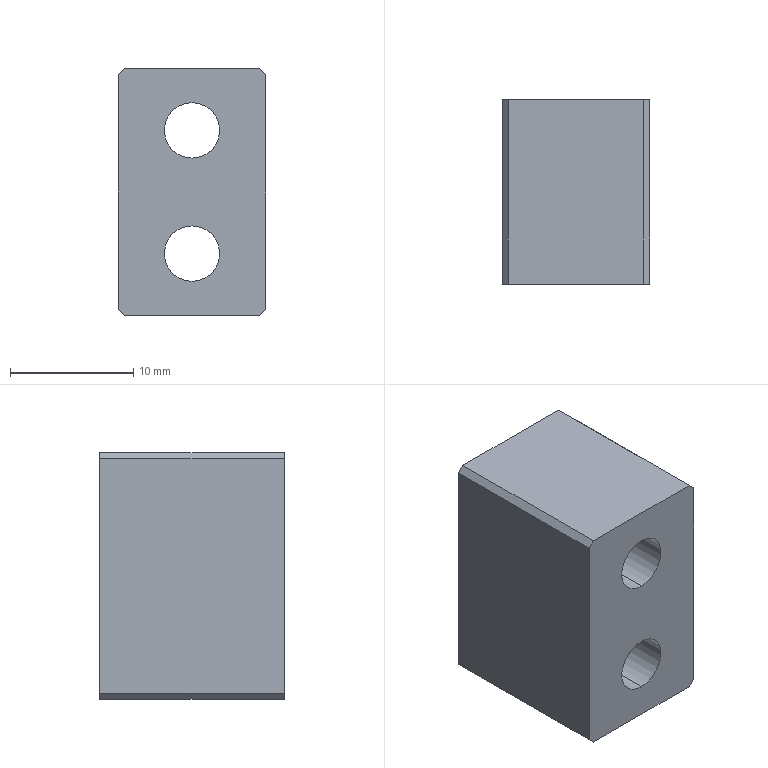Part | SolidWorks | features Chamfer 1, Extrusion 1, HoleWzd 1 | 1 solid | 20 faces | box 12 x 15 x 20 mm | volume 2799 mm3 | plane 12 | cylinder 8 | commonest cylinder face diameters 4.5 x4 8 x4
STEP:
#1=CARTESIAN_POINT('',(0.,10.4,-9.));
#2=VERTEX_POINT('',#1);
#3=CARTESIAN_POINT('',(0.,10.4,-1.));
#4=VERTEX_POINT('',#3);
#5=CARTESIAN_POINT('',(0.,10.4,-5.));
#6=DIRECTION('',(0.,1.,0.));
#7=DIRECTION('',(0.,0.,1.));
#8=AXIS2_PLACEMENT_3D('',#5,#6,#7);
#9=CIRCLE('',#8,4.);
#10=EDGE_CURVE('',#2,#4,#9,.T.);
#11=ORIENTED_EDGE('',*,*,#10,.F.);
#12=CARTESIAN_POINT('',(0.,15.,-9.));
#13=VERTEX_POINT('',#12);
#14=CARTESIAN_POINT('',(0.,15.,-9.));
#15=DIRECTION('',(0.,1.,0.));
#16=VECTOR('',#15,1000.);
#17=LINE('',#14,#16);
#18=EDGE_CURVE('',#2,#13,#17,.T.);
#19=ORIENTED_EDGE('',*,*,#18,.T.);
#20=CARTESIAN_POINT('',(0.,15.,-1.));
#21=VERTEX_POINT('',#20);
#22=CARTESIAN_POINT('',(0.,15.,-5.));
#23=DIRECTION('',(0.,1.,0.));
#24=DIRECTION('',(0.,0.,1.));
#25=AXIS2_PLACEMENT_3D('',#22,#23,#24);
#26=CIRCLE('',#25,4.);
#27=EDGE_CURVE('',#13,#21,#26,.T.);
#28=ORIENTED_EDGE('',*,*,#27,.T.);
#29=CARTESIAN_POINT('',(0.,15.,-1.));
#30=DIRECTION('',(0.,1.,0.));
#31=VECTOR('',#30,1000.);
#32=LINE('',#29,#31);
#33=EDGE_CURVE('',#4,#21,#32,.T.);
#34=ORIENTED_EDGE('',*,*,#33,.F.);
#35=EDGE_LOOP('',(#11,#19,#28,#34));
#36=FACE_OUTER_BOUND('',#35,.T.);
#37=CARTESIAN_POINT('',(0.,15.,-5.));
#38=DIRECTION('',(0.,1.,0.));
#39=DIRECTION('',(0.,0.,1.));
#40=AXIS2_PLACEMENT_3D('',#37,#38,#39);
#41=CYLINDRICAL_SURFACE('',#40,4.);
#42=ADVANCED_FACE('',(#36),#41,.F.);
#43=CARTESIAN_POINT('',(0.,0.,-7.25));
#44=VERTEX_POINT('',#43);
#45=CARTESIAN_POINT('',(0.,0.,-2.75));
#46=VERTEX_POINT('',#45);
#47=CARTESIAN_POINT('',(0.,0.,-5.));
#48=DIRECTION('',(0.,1.,0.));
#49=DIRECTION('',(0.,0.,1.));
#50=AXIS2_PLACEMENT_3D('',#47,#48,#49);
#51=CIRCLE('',#50,2.25);
#52=EDGE_CURVE('',#44,#46,#51,.T.);
#53=ORIENTED_EDGE('',*,*,#52,.F.);
#54=CARTESIAN_POINT('',(0.,10.4,-7.25));
#55=VERTEX_POINT('',#54);
#56=CARTESIAN_POINT('',(0.,15.,-7.25));
#57=DIRECTION('',(0.,1.,0.));
#58=VECTOR('',#57,1000.);
#59=LINE('',#56,#58);
#60=EDGE_CURVE('',#44,#55,#59,.T.);
#61=ORIENTED_EDGE('',*,*,#60,.T.);
#62=CARTESIAN_POINT('',(0.,10.4,-2.75));
#63=VERTEX_POINT('',#62);
#64=CARTESIAN_POINT('',(0.,10.4,-5.));
#65=DIRECTION('',(0.,1.,0.));
#66=DIRECTION('',(0.,0.,1.));
#67=AXIS2_PLACEMENT_3D('',#64,#65,#66);
#68=CIRCLE('',#67,2.25);
#69=EDGE_CURVE('',#55,#63,#68,.T.);
#70=ORIENTED_EDGE('',*,*,#69,.T.);
#71=CARTESIAN_POINT('',(0.,15.,-2.75));
#72=DIRECTION('',(0.,1.,0.));
#73=VECTOR('',#72,1000.);
#74=LINE('',#71,#73);
#75=EDGE_CURVE('',#46,#63,#74,.T.);
#76=ORIENTED_EDGE('',*,*,#75,.F.);
#77=EDGE_LOOP('',(#53,#61,#70,#76));
#78=FACE_OUTER_BOUND('',#77,.T.);
#79=CARTESIAN_POINT('',(0.,15.,-5.));
#80=DIRECTION('',(0.,1.,0.));
#81=DIRECTION('',(0.,0.,1.));
#82=AXIS2_PLACEMENT_3D('',#79,#80,#81);
#83=CYLINDRICAL_SURFACE('',#82,2.25);
#84=ADVANCED_FACE('',(#78),#83,.F.);
#85=CARTESIAN_POINT('',(0.,10.4,1.));
#86=VERTEX_POINT('',#85);
#87=CARTESIAN_POINT('',(0.,10.4,9.));
#88=VERTEX_POINT('',#87);
#89=CARTESIAN_POINT('',(0.,10.4,5.));
#90=DIRECTION('',(0.,1.,0.));
#91=DIRECTION('',(0.,0.,1.));
#92=AXIS2_PLACEMENT_3D('',#89,#90,#91);
#93=CIRCLE('',#92,4.);
#94=EDGE_CURVE('',#86,#88,#93,.T.);
#95=ORIENTED_EDGE('',*,*,#94,.F.);
#96=CARTESIAN_POINT('',(0.,15.,1.));
#97=VERTEX_POINT('',#96);
#98=CARTESIAN_POINT('',(0.,15.,1.));
#99=DIRECTION('',(0.,1.,0.));
#100=VECTOR('',#99,1000.);
#101=LINE('',#98,#100);
#102=EDGE_CURVE('',#86,#97,#101,.T.);
#103=ORIENTED_EDGE('',*,*,#102,.T.);
#104=CARTESIAN_POINT('',(0.,15.,9.));
#105=VERTEX_POINT('',#104);
#106=CARTESIAN_POINT('',(0.,15.,5.));
#107=DIRECTION('',(0.,1.,0.));
#108=DIRECTION('',(0.,0.,1.));
#109=AXIS2_PLACEMENT_3D('',#106,#107,#108);
#110=CIRCLE('',#109,4.);
#111=EDGE_CURVE('',#97,#105,#110,.T.);
#112=ORIENTED_EDGE('',*,*,#111,.T.);
#113=CARTESIAN_POINT('',(0.,15.,9.));
#114=DIRECTION('',(0.,1.,0.));
#115=VECTOR('',#114,1000.);
#116=LINE('',#113,#115);
#117=EDGE_CURVE('',#88,#105,#116,.T.);
#118=ORIENTED_EDGE('',*,*,#117,.F.);
#119=EDGE_LOOP('',(#95,#103,#112,#118));
#120=FACE_OUTER_BOUND('',#119,.T.);
#121=CARTESIAN_POINT('',(0.,15.,5.));
#122=DIRECTION('',(0.,1.,0.));
#123=DIRECTION('',(0.,0.,1.));
#124=AXIS2_PLACEMENT_3D('',#121,#122,#123);
#125=CYLINDRICAL_SURFACE('',#124,4.);
#126=ADVANCED_FACE('',(#120),#125,.F.);
#127=CARTESIAN_POINT('',(0.,0.,2.75));
#128=VERTEX_POINT('',#127);
#129=CARTESIAN_POINT('',(0.,0.,7.25));
#130=VERTEX_POINT('',#129);
#131=CARTESIAN_POINT('',(0.,0.,5.));
#132=DIRECTION('',(0.,1.,0.));
#133=DIRECTION('',(0.,0.,1.));
#134=AXIS2_PLACEMENT_3D('',#131,#132,#133);
#135=CIRCLE('',#134,2.25);
#136=EDGE_CURVE('',#128,#130,#135,.T.);
#137=ORIENTED_EDGE('',*,*,#136,.F.);
#138=CARTESIAN_POINT('',(0.,10.4,2.75));
#139=VERTEX_POINT('',#138);
#140=CARTESIAN_POINT('',(0.,15.,2.75));
#141=DIRECTION('',(0.,1.,0.));
#142=VECTOR('',#141,1000.);
#143=LINE('',#140,#142);
#144=EDGE_CURVE('',#128,#139,#143,.T.);
#145=ORIENTED_EDGE('',*,*,#144,.T.);
#146=CARTESIAN_POINT('',(0.,10.4,7.25));
#147=VERTEX_POINT('',#146);
#148=CARTESIAN_POINT('',(0.,10.4,5.));
#149=DIRECTION('',(0.,1.,0.));
#150=DIRECTION('',(0.,0.,1.));
#151=AXIS2_PLACEMENT_3D('',#148,#149,#150);
#152=CIRCLE('',#151,2.25);
#153=EDGE_CURVE('',#139,#147,#152,.T.);
#154=ORIENTED_EDGE('',*,*,#153,.T.);
#155=CARTESIAN_POINT('',(0.,15.,7.25));
#156=DIRECTION('',(0.,1.,0.));
#157=VECTOR('',#156,1000.);
#158=LINE('',#155,#157);
#159=EDGE_CURVE('',#130,#147,#158,.T.);
#160=ORIENTED_EDGE('',*,*,#159,.F.);
#161=EDGE_LOOP('',(#137,#145,#154,#160));
#162=FACE_OUTER_BOUND('',#161,.T.);
#163=CARTESIAN_POINT('',(0.,15.,5.));
#164=DIRECTION('',(0.,1.,0.));
#165=DIRECTION('',(0.,0.,1.));
#166=AXIS2_PLACEMENT_3D('',#163,#164,#165);
#167=CYLINDRICAL_SURFACE('',#166,2.25);
#168=ADVANCED_FACE('',(#162),#167,.F.);
#169=CARTESIAN_POINT('',(6.,0.,9.5));
#170=VERTEX_POINT('',#169);
#171=CARTESIAN_POINT('',(6.,0.,-9.5));
#172=VERTEX_POINT('',#171);
#173=CARTESIAN_POINT('',(6.,0.,-10.));
#174=DIRECTION('',(0.,0.,-1.));
#175=VECTOR('',#174,1000.);
#176=LINE('',#173,#175);
#177=EDGE_CURVE('',#170,#172,#176,.T.);
#178=ORIENTED_EDGE('',*,*,#177,.T.);
#179=CARTESIAN_POINT('',(6.,15.,-9.5));
#180=VERTEX_POINT('',#179);
#181=CARTESIAN_POINT('',(6.,15.,-9.5));
#182=DIRECTION('',(0.,1.,0.));
#183=VECTOR('',#182,1000.);
#184=LINE('',#181,#183);
#185=EDGE_CURVE('',#172,#180,#184,.T.);
#186=ORIENTED_EDGE('',*,*,#185,.T.);
#187=CARTESIAN_POINT('',(6.,15.,9.5));
#188=VERTEX_POINT('',#187);
#189=CARTESIAN_POINT('',(6.,15.,-10.));
#190=DIRECTION('',(0.,0.,-1.));
#191=VECTOR('',#190,1000.);
#192=LINE('',#189,#191);
#193=EDGE_CURVE('',#188,#180,#192,.T.);
#194=ORIENTED_EDGE('',*,*,#193,.F.);
#195=CARTESIAN_POINT('',(6.,15.,9.5));
#196=DIRECTION('',(0.,-1.,0.));
#197=VECTOR('',#196,1000.);
#198=LINE('',#195,#197);
#199=EDGE_CURVE('',#188,#170,#198,.T.);
#200=ORIENTED_EDGE('',*,*,#199,.T.);
#201=EDGE_LOOP('',(#178,#186,#194,#200));
#202=FACE_OUTER_BOUND('',#201,.T.);
#203=CARTESIAN_POINT('',(6.,15.,-10.));
#204=DIRECTION('',(-1.,0.,0.));
#205=DIRECTION('',(0.,0.,1.));
#206=AXIS2_PLACEMENT_3D('',#203,#204,#205);
#207=PLANE('',#206);
#208=ADVANCED_FACE('',(#202),#207,.F.);
#209=CARTESIAN_POINT('',(5.5,15.,-10.));
#210=VERTEX_POINT('',#209);
#211=CARTESIAN_POINT('',(-5.5,15.,-10.));
#212=VERTEX_POINT('',#211);
#213=CARTESIAN_POINT('',(-6.,15.,-10.));
#214=DIRECTION('',(-1.,0.,0.));
#215=VECTOR('',#214,1000.);
#216=LINE('',#213,#215);
#217=EDGE_CURVE('',#210,#212,#216,.T.);
#218=ORIENTED_EDGE('',*,*,#217,.F.);
#219=CARTESIAN_POINT('',(5.5,0.,-10.));
#220=VERTEX_POINT('',#219);
#221=CARTESIAN_POINT('',(5.5,15.,-10.));
#222=DIRECTION('',(0.,-1.,0.));
#223=VECTOR('',#222,1000.);
#224=LINE('',#221,#223);
#225=EDGE_CURVE('',#210,#220,#224,.T.);
#226=ORIENTED_EDGE('',*,*,#225,.T.);
#227=CARTESIAN_POINT('',(-5.5,0.,-10.));
#228=VERTEX_POINT('',#227);
#229=CARTESIAN_POINT('',(-6.,0.,-10.));
#230=DIRECTION('',(-1.,0.,0.));
#231=VECTOR('',#230,1000.);
#232=LINE('',#229,#231);
#233=EDGE_CURVE('',#220,#228,#232,.T.);
#234=ORIENTED_EDGE('',*,*,#233,.T.);
#235=CARTESIAN_POINT('',(-5.5,15.,-10.));
#236=DIRECTION('',(0.,1.,0.));
#237=VECTOR('',#236,1000.);
#238=LINE('',#235,#237);
#239=EDGE_CURVE('',#228,#212,#238,.T.);
#240=ORIENTED_EDGE('',*,*,#239,.T.);
#241=EDGE_LOOP('',(#218,#226,#234,#240));
#242=FACE_OUTER_BOUND('',#241,.T.);
#243=CARTESIAN_POINT('',(-6.,15.,-10.));
#244=DIRECTION('',(0.,0.,1.));
#245=DIRECTION('',(1.,0.,0.));
#246=AXIS2_PLACEMENT_3D('',#243,#244,#245);
#247=PLANE('',#246);
#248=ADVANCED_FACE('',(#242),#247,.F.);
#249=CARTESIAN_POINT('',(-6.,0.,-9.5));
#250=VERTEX_POINT('',#249);
#251=CARTESIAN_POINT('',(-6.,0.,9.5));
#252=VERTEX_POINT('',#251);
#253=CARTESIAN_POINT('',(-6.,0.,-10.));
#254=DIRECTION('',(0.,0.,1.));
#255=VECTOR('',#254,1000.);
#256=LINE('',#253,#255);
#257=EDGE_CURVE('',#250,#252,#256,.T.);
#258=ORIENTED_EDGE('',*,*,#257,.T.);
#259=CARTESIAN_POINT('',(-6.,15.,9.5));
#260=VERTEX_POINT('',#259);
#261=CARTESIAN_POINT('',(-6.,15.,9.5));
#262=DIRECTION('',(0.,1.,0.));
#263=VECTOR('',#262,1000.);
#264=LINE('',#261,#263);
#265=EDGE_CURVE('',#252,#260,#264,.T.);
#266=ORIENTED_EDGE('',*,*,#265,.T.);
#267=CARTESIAN_POINT('',(-6.,15.,-9.5));
#268=VERTEX_POINT('',#267);
#269=CARTESIAN_POINT('',(-6.,15.,-10.));
#270=DIRECTION('',(0.,0.,1.));
#271=VECTOR('',#270,1000.);
#272=LINE('',#269,#271);
#273=EDGE_CURVE('',#268,#260,#272,.T.);
#274=ORIENTED_EDGE('',*,*,#273,.F.);
#275=CARTESIAN_POINT('',(-6.,15.,-9.5));
#276=DIRECTION('',(0.,-1.,0.));
#277=VECTOR('',#276,1000.);
#278=LINE('',#275,#277);
#279=EDGE_CURVE('',#268,#250,#278,.T.);
#280=ORIENTED_EDGE('',*,*,#279,.T.);
#281=EDGE_LOOP('',(#258,#266,#274,#280));
#282=FACE_OUTER_BOUND('',#281,.T.);
#283=CARTESIAN_POINT('',(-6.,15.,-10.));
#284=DIRECTION('',(1.,0.,0.));
#285=DIRECTION('',(0.,0.,-1.));
#286=AXIS2_PLACEMENT_3D('',#283,#284,#285);
#287=PLANE('',#286);
#288=ADVANCED_FACE('',(#282),#287,.F.);
#289=CARTESIAN_POINT('',(-5.5,0.,10.));
#290=VERTEX_POINT('',#289);
#291=CARTESIAN_POINT('',(5.5,0.,10.));
#292=VERTEX_POINT('',#291);
#293=CARTESIAN_POINT('',(-6.,0.,10.));
#294=DIRECTION('',(1.,0.,0.));
#295=VECTOR('',#294,1000.);
#296=LINE('',#293,#295);
#297=EDGE_CURVE('',#290,#292,#296,.T.);
#298=ORIENTED_EDGE('',*,*,#297,.T.);
#299=CARTESIAN_POINT('',(5.5,15.,10.));
#300=VERTEX_POINT('',#299);
#301=CARTESIAN_POINT('',(5.5,15.,10.));
#302=DIRECTION('',(0.,1.,0.));
#303=VECTOR('',#302,1000.);
#304=LINE('',#301,#303);
#305=EDGE_CURVE('',#292,#300,#304,.T.);
#306=ORIENTED_EDGE('',*,*,#305,.T.);
#307=CARTESIAN_POINT('',(-5.5,15.,10.));
#308=VERTEX_POINT('',#307);
#309=CARTESIAN_POINT('',(-6.,15.,10.));
#310=DIRECTION('',(1.,0.,0.));
#311=VECTOR('',#310,1000.);
#312=LINE('',#309,#311);
#313=EDGE_CURVE('',#308,#300,#312,.T.);
#314=ORIENTED_EDGE('',*,*,#313,.F.);
#315=CARTESIAN_POINT('',(-5.5,15.,10.));
#316=DIRECTION('',(0.,-1.,0.));
#317=VECTOR('',#316,1000.);
#318=LINE('',#315,#317);
#319=EDGE_CURVE('',#308,#290,#318,.T.);
#320=ORIENTED_EDGE('',*,*,#319,.T.);
#321=EDGE_LOOP('',(#298,#306,#314,#320));
#322=FACE_OUTER_BOUND('',#321,.T.);
#323=CARTESIAN_POINT('',(-6.,15.,10.));
#324=DIRECTION('',(0.,0.,-1.));
#325=DIRECTION('',(-1.,0.,0.));
#326=AXIS2_PLACEMENT_3D('',#323,#324,#325);
#327=PLANE('',#326);
#328=ADVANCED_FACE('',(#322),#327,.F.);
#329=CARTESIAN_POINT('',(0.,15.,-5.));
#330=DIRECTION('',(0.,1.,0.));
#331=DIRECTION('',(0.,0.,1.));
#332=AXIS2_PLACEMENT_3D('',#329,#330,#331);
#333=CIRCLE('',#332,4.);
#334=EDGE_CURVE('',#21,#13,#333,.T.);
#335=ORIENTED_EDGE('',*,*,#334,.F.);
#336=ORIENTED_EDGE('',*,*,#27,.F.);
#337=EDGE_LOOP('',(#335,#336));
#338=FACE_BOUND('',#337,.T.);
#339=CARTESIAN_POINT('',(0.,15.,5.));
#340=DIRECTION('',(0.,1.,0.));
#341=DIRECTION('',(0.,0.,1.));
#342=AXIS2_PLACEMENT_3D('',#339,#340,#341);
#343=CIRCLE('',#342,4.);
#344=EDGE_CURVE('',#105,#97,#343,.T.);
#345=ORIENTED_EDGE('',*,*,#344,.F.);
#346=ORIENTED_EDGE('',*,*,#111,.F.);
#347=EDGE_LOOP('',(#345,#346));
#348=FACE_BOUND('',#347,.T.);
#349=ORIENTED_EDGE('',*,*,#193,.T.);
#350=CARTESIAN_POINT('',(7.75,15.,-7.75));
#351=DIRECTION('',(-0.7071,0.,-0.7071));
#352=VECTOR('',#351,1000.);
#353=LINE('',#350,#352);
#354=EDGE_CURVE('',#180,#210,#353,.T.);
#355=ORIENTED_EDGE('',*,*,#354,.T.);
#356=ORIENTED_EDGE('',*,*,#217,.T.);
#357=CARTESIAN_POINT('',(-7.75,15.,-7.75));
#358=DIRECTION('',(-0.7071,0.,0.7071));
#359=VECTOR('',#358,1000.);
#360=LINE('',#357,#359);
#361=EDGE_CURVE('',#212,#268,#360,.T.);
#362=ORIENTED_EDGE('',*,*,#361,.T.);
#363=ORIENTED_EDGE('',*,*,#273,.T.);
#364=CARTESIAN_POINT('',(-7.75,15.,7.75));
#365=DIRECTION('',(0.7071,0.,0.7071));
#366=VECTOR('',#365,1000.);
#367=LINE('',#364,#366);
#368=EDGE_CURVE('',#260,#308,#367,.T.);
#369=ORIENTED_EDGE('',*,*,#368,.T.);
#370=ORIENTED_EDGE('',*,*,#313,.T.);
#371=CARTESIAN_POINT('',(7.75,15.,7.75));
#372=DIRECTION('',(0.7071,0.,-0.7071));
#373=VECTOR('',#372,1000.);
#374=LINE('',#371,#373);
#375=EDGE_CURVE('',#300,#188,#374,.T.);
#376=ORIENTED_EDGE('',*,*,#375,.T.);
#377=EDGE_LOOP('',(#349,#355,#356,#362,#363,#369,#370,#376));
#378=FACE_OUTER_BOUND('',#377,.T.);
#379=CARTESIAN_POINT('',(0.,15.,0.));
#380=DIRECTION('',(0.,1.,0.));
#381=DIRECTION('',(0.,0.,1.));
#382=AXIS2_PLACEMENT_3D('',#379,#380,#381);
#383=PLANE('',#382);
#384=ADVANCED_FACE('',(#338,#348,#378),#383,.T.);
#385=CARTESIAN_POINT('',(0.,0.,-5.));
#386=DIRECTION('',(0.,1.,0.));
#387=DIRECTION('',(0.,0.,1.));
#388=AXIS2_PLACEMENT_3D('',#385,#386,#387);
#389=CIRCLE('',#388,2.25);
#390=EDGE_CURVE('',#46,#44,#389,.T.);
#391=ORIENTED_EDGE('',*,*,#390,.T.);
#392=ORIENTED_EDGE('',*,*,#52,.T.);
#393=EDGE_LOOP('',(#391,#392));
#394=FACE_BOUND('',#393,.T.);
#395=CARTESIAN_POINT('',(0.,0.,5.));
#396=DIRECTION('',(0.,1.,0.));
#397=DIRECTION('',(0.,0.,1.));
#398=AXIS2_PLACEMENT_3D('',#395,#396,#397);
#399=CIRCLE('',#398,2.25);
#400=EDGE_CURVE('',#130,#128,#399,.T.);
#401=ORIENTED_EDGE('',*,*,#400,.T.);
#402=ORIENTED_EDGE('',*,*,#136,.T.);
#403=EDGE_LOOP('',(#401,#402));
#404=FACE_BOUND('',#403,.T.);
#405=ORIENTED_EDGE('',*,*,#233,.F.);
#406=CARTESIAN_POINT('',(5.5,0.,-10.));
#407=DIRECTION('',(0.7071,0.,0.7071));
#408=VECTOR('',#407,1000.);
#409=LINE('',#406,#408);
#410=EDGE_CURVE('',#220,#172,#409,.T.);
#411=ORIENTED_EDGE('',*,*,#410,.T.);
#412=ORIENTED_EDGE('',*,*,#177,.F.);
#413=CARTESIAN_POINT('',(6.,0.,9.5));
#414=DIRECTION('',(-0.7071,0.,0.7071));
#415=VECTOR('',#414,1000.);
#416=LINE('',#413,#415);
#417=EDGE_CURVE('',#170,#292,#416,.T.);
#418=ORIENTED_EDGE('',*,*,#417,.T.);
#419=ORIENTED_EDGE('',*,*,#297,.F.);
#420=CARTESIAN_POINT('',(-5.5,0.,10.));
#421=DIRECTION('',(-0.7071,0.,-0.7071));
#422=VECTOR('',#421,1000.);
#423=LINE('',#420,#422);
#424=EDGE_CURVE('',#290,#252,#423,.T.);
#425=ORIENTED_EDGE('',*,*,#424,.T.);
#426=ORIENTED_EDGE('',*,*,#257,.F.);
#427=CARTESIAN_POINT('',(-6.,0.,-9.5));
#428=DIRECTION('',(0.7071,0.,-0.7071));
#429=VECTOR('',#428,1000.);
#430=LINE('',#427,#429);
#431=EDGE_CURVE('',#250,#228,#430,.T.);
#432=ORIENTED_EDGE('',*,*,#431,.T.);
#433=EDGE_LOOP('',(#405,#411,#412,#418,#419,#425,#426,#432));
#434=FACE_OUTER_BOUND('',#433,.T.);
#435=CARTESIAN_POINT('',(0.,0.,0.));
#436=DIRECTION('',(0.,1.,0.));
#437=DIRECTION('',(0.,0.,1.));
#438=AXIS2_PLACEMENT_3D('',#435,#436,#437);
#439=PLANE('',#438);
#440=ADVANCED_FACE('',(#394,#404,#434),#439,.F.);
#441=ORIENTED_EDGE('',*,*,#144,.F.);
#442=ORIENTED_EDGE('',*,*,#400,.F.);
#443=ORIENTED_EDGE('',*,*,#159,.T.);
#444=CARTESIAN_POINT('',(0.,10.4,5.));
#445=DIRECTION('',(0.,1.,0.));
#446=DIRECTION('',(0.,0.,1.));
#447=AXIS2_PLACEMENT_3D('',#444,#445,#446);
#448=CIRCLE('',#447,2.25);
#449=EDGE_CURVE('',#147,#139,#448,.T.);
#450=ORIENTED_EDGE('',*,*,#449,.T.);
#451=EDGE_LOOP('',(#441,#442,#443,#450));
#452=FACE_OUTER_BOUND('',#451,.T.);
#453=CARTESIAN_POINT('',(0.,15.,5.));
#454=DIRECTION('',(0.,1.,0.));
#455=DIRECTION('',(0.,0.,1.));
#456=AXIS2_PLACEMENT_3D('',#453,#454,#455);
#457=CYLINDRICAL_SURFACE('',#456,2.25);
#458=ADVANCED_FACE('',(#452),#457,.F.);
#459=ORIENTED_EDGE('',*,*,#449,.F.);
#460=ORIENTED_EDGE('',*,*,#153,.F.);
#461=EDGE_LOOP('',(#459,#460));
#462=FACE_BOUND('',#461,.T.);
#463=CARTESIAN_POINT('',(0.,10.4,5.));
#464=DIRECTION('',(0.,1.,0.));
#465=DIRECTION('',(0.,0.,1.));
#466=AXIS2_PLACEMENT_3D('',#463,#464,#465);
#467=CIRCLE('',#466,4.);
#468=EDGE_CURVE('',#88,#86,#467,.T.);
#469=ORIENTED_EDGE('',*,*,#468,.T.);
#470=ORIENTED_EDGE('',*,*,#94,.T.);
#471=EDGE_LOOP('',(#469,#470));
#472=FACE_OUTER_BOUND('',#471,.T.);
#473=CARTESIAN_POINT('',(2.25,10.4,5.));
#474=DIRECTION('',(0.,-1.,0.));
#475=DIRECTION('',(0.,0.,-1.));
#476=AXIS2_PLACEMENT_3D('',#473,#474,#475);
#477=PLANE('',#476);
#478=ADVANCED_FACE('',(#462,#472),#477,.F.);
#479=ORIENTED_EDGE('',*,*,#102,.F.);
#480=ORIENTED_EDGE('',*,*,#468,.F.);
#481=ORIENTED_EDGE('',*,*,#117,.T.);
#482=ORIENTED_EDGE('',*,*,#344,.T.);
#483=EDGE_LOOP('',(#479,#480,#481,#482));
#484=FACE_OUTER_BOUND('',#483,.T.);
#485=CARTESIAN_POINT('',(0.,15.,5.));
#486=DIRECTION('',(0.,1.,0.));
#487=DIRECTION('',(0.,0.,1.));
#488=AXIS2_PLACEMENT_3D('',#485,#486,#487);
#489=CYLINDRICAL_SURFACE('',#488,4.);
#490=ADVANCED_FACE('',(#484),#489,.F.);
#491=ORIENTED_EDGE('',*,*,#60,.F.);
#492=ORIENTED_EDGE('',*,*,#390,.F.);
#493=ORIENTED_EDGE('',*,*,#75,.T.);
#494=CARTESIAN_POINT('',(0.,10.4,-5.));
#495=DIRECTION('',(0.,1.,0.));
#496=DIRECTION('',(0.,0.,1.));
#497=AXIS2_PLACEMENT_3D('',#494,#495,#496);
#498=CIRCLE('',#497,2.25);
#499=EDGE_CURVE('',#63,#55,#498,.T.);
#500=ORIENTED_EDGE('',*,*,#499,.T.);
#501=EDGE_LOOP('',(#491,#492,#493,#500));
#502=FACE_OUTER_BOUND('',#501,.T.);
#503=CARTESIAN_POINT('',(0.,15.,-5.));
#504=DIRECTION('',(0.,1.,0.));
#505=DIRECTION('',(0.,0.,1.));
#506=AXIS2_PLACEMENT_3D('',#503,#504,#505);
#507=CYLINDRICAL_SURFACE('',#506,2.25);
#508=ADVANCED_FACE('',(#502),#507,.F.);
#509=ORIENTED_EDGE('',*,*,#499,.F.);
#510=ORIENTED_EDGE('',*,*,#69,.F.);
#511=EDGE_LOOP('',(#509,#510));
#512=FACE_BOUND('',#511,.T.);
#513=CARTESIAN_POINT('',(0.,10.4,-5.));
#514=DIRECTION('',(0.,1.,0.));
#515=DIRECTION('',(0.,0.,1.));
#516=AXIS2_PLACEMENT_3D('',#513,#514,#515);
#517=CIRCLE('',#516,4.);
#518=EDGE_CURVE('',#4,#2,#517,.T.);
#519=ORIENTED_EDGE('',*,*,#518,.T.);
#520=ORIENTED_EDGE('',*,*,#10,.T.);
#521=EDGE_LOOP('',(#519,#520));
#522=FACE_OUTER_BOUND('',#521,.T.);
#523=CARTESIAN_POINT('',(2.25,10.4,-5.));
#524=DIRECTION('',(0.,-1.,0.));
#525=DIRECTION('',(0.,0.,-1.));
#526=AXIS2_PLACEMENT_3D('',#523,#524,#525);
#527=PLANE('',#526);
#528=ADVANCED_FACE('',(#512,#522),#527,.F.);
#529=ORIENTED_EDGE('',*,*,#18,.F.);
#530=ORIENTED_EDGE('',*,*,#518,.F.);
#531=ORIENTED_EDGE('',*,*,#33,.T.);
#532=ORIENTED_EDGE('',*,*,#334,.T.);
#533=EDGE_LOOP('',(#529,#530,#531,#532));
#534=FACE_OUTER_BOUND('',#533,.T.);
#535=CARTESIAN_POINT('',(0.,15.,-5.));
#536=DIRECTION('',(0.,1.,0.));
#537=DIRECTION('',(0.,0.,1.));
#538=AXIS2_PLACEMENT_3D('',#535,#536,#537);
#539=CYLINDRICAL_SURFACE('',#538,4.);
#540=ADVANCED_FACE('',(#534),#539,.F.);
#541=ORIENTED_EDGE('',*,*,#354,.F.);
#542=ORIENTED_EDGE('',*,*,#185,.F.);
#543=ORIENTED_EDGE('',*,*,#410,.F.);
#544=ORIENTED_EDGE('',*,*,#225,.F.);
#545=EDGE_LOOP('',(#541,#542,#543,#544));
#546=FACE_OUTER_BOUND('',#545,.T.);
#547=CARTESIAN_POINT('',(5.5,15.,-10.));
#548=DIRECTION('',(-0.7071,0.,0.7071));
#549=DIRECTION('',(0.,-1.,0.));
#550=AXIS2_PLACEMENT_3D('',#547,#548,#549);
#551=PLANE('',#550);
#552=ADVANCED_FACE('',(#546),#551,.F.);
#553=ORIENTED_EDGE('',*,*,#375,.F.);
#554=ORIENTED_EDGE('',*,*,#305,.F.);
#555=ORIENTED_EDGE('',*,*,#417,.F.);
#556=ORIENTED_EDGE('',*,*,#199,.F.);
#557=EDGE_LOOP('',(#553,#554,#555,#556));
#558=FACE_OUTER_BOUND('',#557,.T.);
#559=CARTESIAN_POINT('',(6.,15.,9.5));
#560=DIRECTION('',(-0.7071,0.,-0.7071));
#561=DIRECTION('',(0.,-1.,0.));
#562=AXIS2_PLACEMENT_3D('',#559,#560,#561);
#563=PLANE('',#562);
#564=ADVANCED_FACE('',(#558),#563,.F.);
#565=ORIENTED_EDGE('',*,*,#368,.F.);
#566=ORIENTED_EDGE('',*,*,#265,.F.);
#567=ORIENTED_EDGE('',*,*,#424,.F.);
#568=ORIENTED_EDGE('',*,*,#319,.F.);
#569=EDGE_LOOP('',(#565,#566,#567,#568));
#570=FACE_OUTER_BOUND('',#569,.T.);
#571=CARTESIAN_POINT('',(-5.5,15.,10.));
#572=DIRECTION('',(0.7071,0.,-0.7071));
#573=DIRECTION('',(0.,-1.,0.));
#574=AXIS2_PLACEMENT_3D('',#571,#572,#573);
#575=PLANE('',#574);
#576=ADVANCED_FACE('',(#570),#575,.F.);
#577=ORIENTED_EDGE('',*,*,#361,.F.);
#578=ORIENTED_EDGE('',*,*,#239,.F.);
#579=ORIENTED_EDGE('',*,*,#431,.F.);
#580=ORIENTED_EDGE('',*,*,#279,.F.);
#581=EDGE_LOOP('',(#577,#578,#579,#580));
#582=FACE_OUTER_BOUND('',#581,.T.);
#583=CARTESIAN_POINT('',(-6.,15.,-9.5));
#584=DIRECTION('',(0.7071,0.,0.7071));
#585=DIRECTION('',(0.,-1.,0.));
#586=AXIS2_PLACEMENT_3D('',#583,#584,#585);
#587=PLANE('',#586);
#588=ADVANCED_FACE('',(#582),#587,.F.);
#589=CLOSED_SHELL('',(#42,#84,#126,#168,#208,#248,#288,#328,#384,#440,#458,#478,#490,#508,#528,#540,#552,#564,#576,#588));
#590=MANIFOLD_SOLID_BREP('',#589);
#591=CARTESIAN_POINT('',(0.,0.,0.));
#592=DIRECTION('',(0.,0.,1.));
#593=DIRECTION('',(1.,0.,0.));
#594=AXIS2_PLACEMENT_3D('',#591,#592,#593);
#595=(LENGTH_UNIT()NAMED_UNIT(*)SI_UNIT(.MILLI.,.METRE.));
#596=UNCERTAINTY_MEASURE_WITH_UNIT(LENGTH_MEASURE(0.00001),#595,'','');
#597=(NAMED_UNIT(*)PLANE_ANGLE_UNIT()SI_UNIT($,.RADIAN.));
#598=(NAMED_UNIT(*)SI_UNIT($,.STERADIAN.)SOLID_ANGLE_UNIT());
#599=(GEOMETRIC_REPRESENTATION_CONTEXT(3)GLOBAL_UNCERTAINTY_ASSIGNED_CONTEXT((#596))GLOBAL_UNIT_ASSIGNED_CONTEXT((#595,#597,#598))REPRESENTATION_CONTEXT('',''));
#600=ADVANCED_BREP_SHAPE_REPRESENTATION('',(#590,#594),#599);